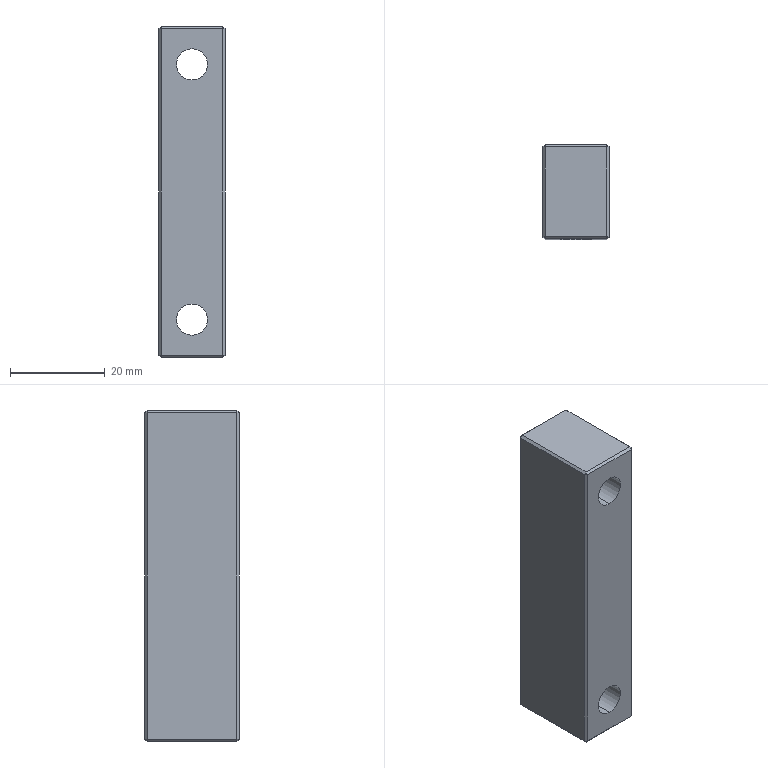Part | STEP file | OP10-116_work-guide | 1 solid | 40 faces | box 14 x 20 x 70 mm | volume 17393 mm3 | plane 28 | cylinder 8 | cone 4 | commonest cylinder face diameters 6.6 x4 11 x4